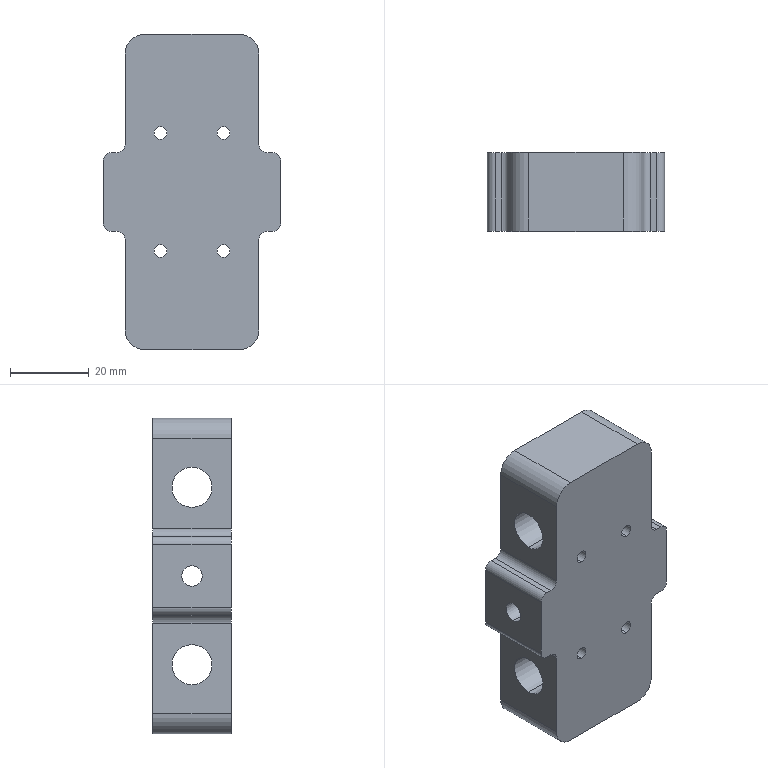Part | SolidWorks | features BaseBody 1 | 1 solid | 40 faces | box 45 x 20 x 80 mm | volume 51215 mm3 | cylinder 26 | plane 14 | commonest cylinder face diameters 3.2 x8 4 x8 10 x4 10.2 x4 5.2 x2
STEP:
#1=CARTESIAN_POINT('',(8.,20.,13.4));
#2=VERTEX_POINT('',#1);
#3=CARTESIAN_POINT('',(8.,20.,16.6));
#4=VERTEX_POINT('',#3);
#5=CARTESIAN_POINT('',(8.,20.,15.));
#6=DIRECTION('',(0.,1.,0.));
#7=DIRECTION('',(0.,0.,-1.));
#8=AXIS2_PLACEMENT_3D('',#5,#6,#7);
#9=CIRCLE('',#8,1.6);
#10=EDGE_CURVE('',#2,#4,#9,.T.);
#11=ORIENTED_EDGE('',*,*,#10,.T.);
#12=CARTESIAN_POINT('',(8.,0.,16.6));
#13=VERTEX_POINT('',#12);
#14=CARTESIAN_POINT('',(8.,20.,16.6));
#15=DIRECTION('',(0.,-1.,0.));
#16=VECTOR('',#15,1000.);
#17=LINE('',#14,#16);
#18=EDGE_CURVE('',#4,#13,#17,.T.);
#19=ORIENTED_EDGE('',*,*,#18,.T.);
#20=CARTESIAN_POINT('',(8.,0.,13.4));
#21=VERTEX_POINT('',#20);
#22=CARTESIAN_POINT('',(8.,0.,15.));
#23=DIRECTION('',(0.,1.,0.));
#24=DIRECTION('',(0.,0.,-1.));
#25=AXIS2_PLACEMENT_3D('',#22,#23,#24);
#26=CIRCLE('',#25,1.6);
#27=EDGE_CURVE('',#21,#13,#26,.T.);
#28=ORIENTED_EDGE('',*,*,#27,.F.);
#29=CARTESIAN_POINT('',(8.,20.,13.4));
#30=DIRECTION('',(0.,-1.,0.));
#31=VECTOR('',#30,1000.);
#32=LINE('',#29,#31);
#33=EDGE_CURVE('',#2,#21,#32,.T.);
#34=ORIENTED_EDGE('',*,*,#33,.F.);
#35=EDGE_LOOP('',(#11,#19,#28,#34));
#36=FACE_OUTER_BOUND('',#35,.T.);
#37=CARTESIAN_POINT('',(8.,20.,15.));
#38=DIRECTION('',(0.,-1.,0.));
#39=DIRECTION('',(0.,0.,-1.));
#40=AXIS2_PLACEMENT_3D('',#37,#38,#39);
#41=CYLINDRICAL_SURFACE('',#40,1.6);
#42=ADVANCED_FACE('',(#36),#41,.F.);
#43=CARTESIAN_POINT('',(-8.,20.,13.4));
#44=VERTEX_POINT('',#43);
#45=CARTESIAN_POINT('',(-8.,20.,16.6));
#46=VERTEX_POINT('',#45);
#47=CARTESIAN_POINT('',(-8.,20.,15.));
#48=DIRECTION('',(0.,1.,0.));
#49=DIRECTION('',(0.,0.,-1.));
#50=AXIS2_PLACEMENT_3D('',#47,#48,#49);
#51=CIRCLE('',#50,1.6);
#52=EDGE_CURVE('',#44,#46,#51,.T.);
#53=ORIENTED_EDGE('',*,*,#52,.T.);
#54=CARTESIAN_POINT('',(-8.,0.,16.6));
#55=VERTEX_POINT('',#54);
#56=CARTESIAN_POINT('',(-8.,20.,16.6));
#57=DIRECTION('',(0.,-1.,0.));
#58=VECTOR('',#57,1000.);
#59=LINE('',#56,#58);
#60=EDGE_CURVE('',#46,#55,#59,.T.);
#61=ORIENTED_EDGE('',*,*,#60,.T.);
#62=CARTESIAN_POINT('',(-8.,0.,13.4));
#63=VERTEX_POINT('',#62);
#64=CARTESIAN_POINT('',(-8.,0.,15.));
#65=DIRECTION('',(0.,1.,0.));
#66=DIRECTION('',(0.,0.,-1.));
#67=AXIS2_PLACEMENT_3D('',#64,#65,#66);
#68=CIRCLE('',#67,1.6);
#69=EDGE_CURVE('',#63,#55,#68,.T.);
#70=ORIENTED_EDGE('',*,*,#69,.F.);
#71=CARTESIAN_POINT('',(-8.,20.,13.4));
#72=DIRECTION('',(0.,-1.,0.));
#73=VECTOR('',#72,1000.);
#74=LINE('',#71,#73);
#75=EDGE_CURVE('',#44,#63,#74,.T.);
#76=ORIENTED_EDGE('',*,*,#75,.F.);
#77=EDGE_LOOP('',(#53,#61,#70,#76));
#78=FACE_OUTER_BOUND('',#77,.T.);
#79=CARTESIAN_POINT('',(-8.,20.,15.));
#80=DIRECTION('',(0.,-1.,0.));
#81=DIRECTION('',(0.,0.,-1.));
#82=AXIS2_PLACEMENT_3D('',#79,#80,#81);
#83=CYLINDRICAL_SURFACE('',#82,1.6);
#84=ADVANCED_FACE('',(#78),#83,.F.);
#85=CARTESIAN_POINT('',(-8.,20.,-16.6));
#86=VERTEX_POINT('',#85);
#87=CARTESIAN_POINT('',(-8.,20.,-13.4));
#88=VERTEX_POINT('',#87);
#89=CARTESIAN_POINT('',(-8.,20.,-15.));
#90=DIRECTION('',(0.,1.,0.));
#91=DIRECTION('',(0.,0.,-1.));
#92=AXIS2_PLACEMENT_3D('',#89,#90,#91);
#93=CIRCLE('',#92,1.6);
#94=EDGE_CURVE('',#86,#88,#93,.T.);
#95=ORIENTED_EDGE('',*,*,#94,.T.);
#96=CARTESIAN_POINT('',(-8.,0.,-13.4));
#97=VERTEX_POINT('',#96);
#98=CARTESIAN_POINT('',(-8.,20.,-13.4));
#99=DIRECTION('',(0.,-1.,0.));
#100=VECTOR('',#99,1000.);
#101=LINE('',#98,#100);
#102=EDGE_CURVE('',#88,#97,#101,.T.);
#103=ORIENTED_EDGE('',*,*,#102,.T.);
#104=CARTESIAN_POINT('',(-8.,0.,-16.6));
#105=VERTEX_POINT('',#104);
#106=CARTESIAN_POINT('',(-8.,0.,-15.));
#107=DIRECTION('',(0.,1.,0.));
#108=DIRECTION('',(0.,0.,-1.));
#109=AXIS2_PLACEMENT_3D('',#106,#107,#108);
#110=CIRCLE('',#109,1.6);
#111=EDGE_CURVE('',#105,#97,#110,.T.);
#112=ORIENTED_EDGE('',*,*,#111,.F.);
#113=CARTESIAN_POINT('',(-8.,20.,-16.6));
#114=DIRECTION('',(0.,-1.,0.));
#115=VECTOR('',#114,1000.);
#116=LINE('',#113,#115);
#117=EDGE_CURVE('',#86,#105,#116,.T.);
#118=ORIENTED_EDGE('',*,*,#117,.F.);
#119=EDGE_LOOP('',(#95,#103,#112,#118));
#120=FACE_OUTER_BOUND('',#119,.T.);
#121=CARTESIAN_POINT('',(-8.,20.,-15.));
#122=DIRECTION('',(0.,-1.,0.));
#123=DIRECTION('',(0.,0.,-1.));
#124=AXIS2_PLACEMENT_3D('',#121,#122,#123);
#125=CYLINDRICAL_SURFACE('',#124,1.6);
#126=ADVANCED_FACE('',(#120),#125,.F.);
#127=CARTESIAN_POINT('',(8.,20.,-16.6));
#128=VERTEX_POINT('',#127);
#129=CARTESIAN_POINT('',(8.,20.,-13.4));
#130=VERTEX_POINT('',#129);
#131=CARTESIAN_POINT('',(8.,20.,-15.));
#132=DIRECTION('',(0.,1.,0.));
#133=DIRECTION('',(0.,0.,-1.));
#134=AXIS2_PLACEMENT_3D('',#131,#132,#133);
#135=CIRCLE('',#134,1.6);
#136=EDGE_CURVE('',#128,#130,#135,.T.);
#137=ORIENTED_EDGE('',*,*,#136,.T.);
#138=CARTESIAN_POINT('',(8.,0.,-13.4));
#139=VERTEX_POINT('',#138);
#140=CARTESIAN_POINT('',(8.,20.,-13.4));
#141=DIRECTION('',(0.,-1.,0.));
#142=VECTOR('',#141,1000.);
#143=LINE('',#140,#142);
#144=EDGE_CURVE('',#130,#139,#143,.T.);
#145=ORIENTED_EDGE('',*,*,#144,.T.);
#146=CARTESIAN_POINT('',(8.,0.,-16.6));
#147=VERTEX_POINT('',#146);
#148=CARTESIAN_POINT('',(8.,0.,-15.));
#149=DIRECTION('',(0.,1.,0.));
#150=DIRECTION('',(0.,0.,-1.));
#151=AXIS2_PLACEMENT_3D('',#148,#149,#150);
#152=CIRCLE('',#151,1.6);
#153=EDGE_CURVE('',#147,#139,#152,.T.);
#154=ORIENTED_EDGE('',*,*,#153,.F.);
#155=CARTESIAN_POINT('',(8.,20.,-16.6));
#156=DIRECTION('',(0.,-1.,0.));
#157=VECTOR('',#156,1000.);
#158=LINE('',#155,#157);
#159=EDGE_CURVE('',#128,#147,#158,.T.);
#160=ORIENTED_EDGE('',*,*,#159,.F.);
#161=EDGE_LOOP('',(#137,#145,#154,#160));
#162=FACE_OUTER_BOUND('',#161,.T.);
#163=CARTESIAN_POINT('',(8.,20.,-15.));
#164=DIRECTION('',(0.,-1.,0.));
#165=DIRECTION('',(0.,0.,-1.));
#166=AXIS2_PLACEMENT_3D('',#163,#164,#165);
#167=CYLINDRICAL_SURFACE('',#166,1.6);
#168=ADVANCED_FACE('',(#162),#167,.F.);
#169=CARTESIAN_POINT('',(17.,10.,-17.4));
#170=VERTEX_POINT('',#169);
#171=CARTESIAN_POINT('',(17.,10.,-27.6));
#172=VERTEX_POINT('',#171);
#173=CARTESIAN_POINT('',(17.,10.,-22.5));
#174=DIRECTION('',(1.,0.,0.));
#175=DIRECTION('',(0.,0.,1.));
#176=AXIS2_PLACEMENT_3D('',#173,#174,#175);
#177=CIRCLE('',#176,5.1);
#178=EDGE_CURVE('',#170,#172,#177,.T.);
#179=ORIENTED_EDGE('',*,*,#178,.T.);
#180=CARTESIAN_POINT('',(-17.,10.,-27.6));
#181=VERTEX_POINT('',#180);
#182=CARTESIAN_POINT('',(22.5,10.,-27.6));
#183=DIRECTION('',(-1.,0.,0.));
#184=VECTOR('',#183,1000.);
#185=LINE('',#182,#184);
#186=EDGE_CURVE('',#172,#181,#185,.T.);
#187=ORIENTED_EDGE('',*,*,#186,.T.);
#188=CARTESIAN_POINT('',(-17.,10.,-17.4));
#189=VERTEX_POINT('',#188);
#190=CARTESIAN_POINT('',(-17.,10.,-22.5));
#191=DIRECTION('',(-1.,0.,0.));
#192=DIRECTION('',(0.,0.,1.));
#193=AXIS2_PLACEMENT_3D('',#190,#191,#192);
#194=CIRCLE('',#193,5.1);
#195=EDGE_CURVE('',#181,#189,#194,.T.);
#196=ORIENTED_EDGE('',*,*,#195,.T.);
#197=CARTESIAN_POINT('',(22.5,10.,-17.4));
#198=DIRECTION('',(-1.,0.,0.));
#199=VECTOR('',#198,1000.);
#200=LINE('',#197,#199);
#201=EDGE_CURVE('',#170,#189,#200,.T.);
#202=ORIENTED_EDGE('',*,*,#201,.F.);
#203=EDGE_LOOP('',(#179,#187,#196,#202));
#204=FACE_OUTER_BOUND('',#203,.T.);
#205=CARTESIAN_POINT('',(22.5,10.,-22.5));
#206=DIRECTION('',(-1.,0.,0.));
#207=DIRECTION('',(0.,0.,1.));
#208=AXIS2_PLACEMENT_3D('',#205,#206,#207);
#209=CYLINDRICAL_SURFACE('',#208,5.1);
#210=ADVANCED_FACE('',(#204),#209,.F.);
#211=CARTESIAN_POINT('',(22.5,10.,2.6));
#212=VERTEX_POINT('',#211);
#213=CARTESIAN_POINT('',(22.5,10.,-2.6));
#214=VERTEX_POINT('',#213);
#215=CARTESIAN_POINT('',(22.5,10.,0.));
#216=DIRECTION('',(1.,0.,0.));
#217=DIRECTION('',(0.,0.,1.));
#218=AXIS2_PLACEMENT_3D('',#215,#216,#217);
#219=CIRCLE('',#218,2.6);
#220=EDGE_CURVE('',#212,#214,#219,.T.);
#221=ORIENTED_EDGE('',*,*,#220,.T.);
#222=CARTESIAN_POINT('',(-22.5,10.,-2.6));
#223=VERTEX_POINT('',#222);
#224=CARTESIAN_POINT('',(22.5,10.,-2.6));
#225=DIRECTION('',(-1.,0.,0.));
#226=VECTOR('',#225,1000.);
#227=LINE('',#224,#226);
#228=EDGE_CURVE('',#214,#223,#227,.T.);
#229=ORIENTED_EDGE('',*,*,#228,.T.);
#230=CARTESIAN_POINT('',(-22.5,10.,2.6));
#231=VERTEX_POINT('',#230);
#232=CARTESIAN_POINT('',(-22.5,10.,0.));
#233=DIRECTION('',(-1.,0.,0.));
#234=DIRECTION('',(0.,0.,1.));
#235=AXIS2_PLACEMENT_3D('',#232,#233,#234);
#236=CIRCLE('',#235,2.6);
#237=EDGE_CURVE('',#223,#231,#236,.T.);
#238=ORIENTED_EDGE('',*,*,#237,.T.);
#239=CARTESIAN_POINT('',(22.5,10.,2.6));
#240=DIRECTION('',(-1.,0.,0.));
#241=VECTOR('',#240,1000.);
#242=LINE('',#239,#241);
#243=EDGE_CURVE('',#212,#231,#242,.T.);
#244=ORIENTED_EDGE('',*,*,#243,.F.);
#245=EDGE_LOOP('',(#221,#229,#238,#244));
#246=FACE_OUTER_BOUND('',#245,.T.);
#247=CARTESIAN_POINT('',(22.5,10.,0.));
#248=DIRECTION('',(-1.,0.,0.));
#249=DIRECTION('',(0.,0.,1.));
#250=AXIS2_PLACEMENT_3D('',#247,#248,#249);
#251=CYLINDRICAL_SURFACE('',#250,2.6);
#252=ADVANCED_FACE('',(#246),#251,.F.);
#253=CARTESIAN_POINT('',(17.,10.,27.6));
#254=VERTEX_POINT('',#253);
#255=CARTESIAN_POINT('',(17.,10.,17.4));
#256=VERTEX_POINT('',#255);
#257=CARTESIAN_POINT('',(17.,10.,22.5));
#258=DIRECTION('',(1.,0.,0.));
#259=DIRECTION('',(0.,0.,1.));
#260=AXIS2_PLACEMENT_3D('',#257,#258,#259);
#261=CIRCLE('',#260,5.1);
#262=EDGE_CURVE('',#254,#256,#261,.T.);
#263=ORIENTED_EDGE('',*,*,#262,.T.);
#264=CARTESIAN_POINT('',(-17.,10.,17.4));
#265=VERTEX_POINT('',#264);
#266=CARTESIAN_POINT('',(22.5,10.,17.4));
#267=DIRECTION('',(-1.,0.,0.));
#268=VECTOR('',#267,1000.);
#269=LINE('',#266,#268);
#270=EDGE_CURVE('',#256,#265,#269,.T.);
#271=ORIENTED_EDGE('',*,*,#270,.T.);
#272=CARTESIAN_POINT('',(-17.,10.,27.6));
#273=VERTEX_POINT('',#272);
#274=CARTESIAN_POINT('',(-17.,10.,22.5));
#275=DIRECTION('',(-1.,0.,0.));
#276=DIRECTION('',(0.,0.,1.));
#277=AXIS2_PLACEMENT_3D('',#274,#275,#276);
#278=CIRCLE('',#277,5.1);
#279=EDGE_CURVE('',#265,#273,#278,.T.);
#280=ORIENTED_EDGE('',*,*,#279,.T.);
#281=CARTESIAN_POINT('',(22.5,10.,27.6));
#282=DIRECTION('',(-1.,0.,0.));
#283=VECTOR('',#282,1000.);
#284=LINE('',#281,#283);
#285=EDGE_CURVE('',#254,#273,#284,.T.);
#286=ORIENTED_EDGE('',*,*,#285,.F.);
#287=EDGE_LOOP('',(#263,#271,#280,#286));
#288=FACE_OUTER_BOUND('',#287,.T.);
#289=CARTESIAN_POINT('',(22.5,10.,22.5));
#290=DIRECTION('',(-1.,0.,0.));
#291=DIRECTION('',(0.,0.,1.));
#292=AXIS2_PLACEMENT_3D('',#289,#290,#291);
#293=CYLINDRICAL_SURFACE('',#292,5.1);
#294=ADVANCED_FACE('',(#288),#293,.F.);
#295=CARTESIAN_POINT('',(12.,20.,-40.));
#296=VERTEX_POINT('',#295);
#297=CARTESIAN_POINT('',(17.,20.,-35.));
#298=VERTEX_POINT('',#297);
#299=CARTESIAN_POINT('',(12.,20.,-35.));
#300=DIRECTION('',(0.,-1.,0.));
#301=DIRECTION('',(0.,0.,1.));
#302=AXIS2_PLACEMENT_3D('',#299,#300,#301);
#303=CIRCLE('',#302,5.);
#304=EDGE_CURVE('',#296,#298,#303,.T.);
#305=ORIENTED_EDGE('',*,*,#304,.F.);
#306=CARTESIAN_POINT('',(-12.,20.,-40.));
#307=VERTEX_POINT('',#306);
#308=CARTESIAN_POINT('',(0.,20.,-40.));
#309=DIRECTION('',(1.,0.,0.));
#310=VECTOR('',#309,1000.);
#311=LINE('',#308,#310);
#312=EDGE_CURVE('',#307,#296,#311,.T.);
#313=ORIENTED_EDGE('',*,*,#312,.F.);
#314=CARTESIAN_POINT('',(-17.,20.,-35.));
#315=VERTEX_POINT('',#314);
#316=CARTESIAN_POINT('',(-12.,20.,-35.));
#317=DIRECTION('',(0.,-1.,0.));
#318=DIRECTION('',(0.,0.,1.));
#319=AXIS2_PLACEMENT_3D('',#316,#317,#318);
#320=CIRCLE('',#319,5.);
#321=EDGE_CURVE('',#315,#307,#320,.T.);
#322=ORIENTED_EDGE('',*,*,#321,.F.);
#323=CARTESIAN_POINT('',(-17.,20.,-12.));
#324=VERTEX_POINT('',#323);
#325=CARTESIAN_POINT('',(-17.,20.,0.));
#326=DIRECTION('',(0.,0.,-1.));
#327=VECTOR('',#326,1000.);
#328=LINE('',#325,#327);
#329=EDGE_CURVE('',#324,#315,#328,.T.);
#330=ORIENTED_EDGE('',*,*,#329,.F.);
#331=CARTESIAN_POINT('',(-19.,20.,-10.));
#332=VERTEX_POINT('',#331);
#333=CARTESIAN_POINT('',(-19.,20.,-12.));
#334=DIRECTION('',(0.,1.,0.));
#335=DIRECTION('',(0.,0.,-1.));
#336=AXIS2_PLACEMENT_3D('',#333,#334,#335);
#337=CIRCLE('',#336,2.);
#338=EDGE_CURVE('',#332,#324,#337,.T.);
#339=ORIENTED_EDGE('',*,*,#338,.F.);
#340=CARTESIAN_POINT('',(-20.5,20.,-10.));
#341=VERTEX_POINT('',#340);
#342=CARTESIAN_POINT('',(-17.,20.,-10.));
#343=DIRECTION('',(1.,0.,0.));
#344=VECTOR('',#343,1000.);
#345=LINE('',#342,#344);
#346=EDGE_CURVE('',#341,#332,#345,.T.);
#347=ORIENTED_EDGE('',*,*,#346,.F.);
#348=CARTESIAN_POINT('',(-22.5,20.,-8.));
#349=VERTEX_POINT('',#348);
#350=CARTESIAN_POINT('',(-20.5,20.,-8.));
#351=DIRECTION('',(0.,-1.,0.));
#352=DIRECTION('',(0.,0.,1.));
#353=AXIS2_PLACEMENT_3D('',#350,#351,#352);
#354=CIRCLE('',#353,2.);
#355=EDGE_CURVE('',#349,#341,#354,.T.);
#356=ORIENTED_EDGE('',*,*,#355,.F.);
#357=CARTESIAN_POINT('',(-22.5,20.,8.));
#358=VERTEX_POINT('',#357);
#359=CARTESIAN_POINT('',(-22.5,20.,0.));
#360=DIRECTION('',(0.,0.,-1.));
#361=VECTOR('',#360,1000.);
#362=LINE('',#359,#361);
#363=EDGE_CURVE('',#358,#349,#362,.T.);
#364=ORIENTED_EDGE('',*,*,#363,.F.);
#365=CARTESIAN_POINT('',(-20.5,20.,10.));
#366=VERTEX_POINT('',#365);
#367=CARTESIAN_POINT('',(-20.5,20.,8.));
#368=DIRECTION('',(0.,-1.,0.));
#369=DIRECTION('',(0.,0.,-1.));
#370=AXIS2_PLACEMENT_3D('',#367,#368,#369);
#371=CIRCLE('',#370,2.);
#372=EDGE_CURVE('',#366,#358,#371,.T.);
#373=ORIENTED_EDGE('',*,*,#372,.F.);
#374=CARTESIAN_POINT('',(-19.,20.,10.));
#375=VERTEX_POINT('',#374);
#376=CARTESIAN_POINT('',(-17.,20.,10.));
#377=DIRECTION('',(1.,0.,0.));
#378=VECTOR('',#377,1000.);
#379=LINE('',#376,#378);
#380=EDGE_CURVE('',#366,#375,#379,.T.);
#381=ORIENTED_EDGE('',*,*,#380,.T.);
#382=CARTESIAN_POINT('',(-17.,20.,12.));
#383=VERTEX_POINT('',#382);
#384=CARTESIAN_POINT('',(-19.,20.,12.));
#385=DIRECTION('',(0.,1.,0.));
#386=DIRECTION('',(0.,0.,1.));
#387=AXIS2_PLACEMENT_3D('',#384,#385,#386);
#388=CIRCLE('',#387,2.);
#389=EDGE_CURVE('',#383,#375,#388,.T.);
#390=ORIENTED_EDGE('',*,*,#389,.F.);
#391=CARTESIAN_POINT('',(-17.,20.,35.));
#392=VERTEX_POINT('',#391);
#393=CARTESIAN_POINT('',(-17.,20.,0.));
#394=DIRECTION('',(0.,0.,-1.));
#395=VECTOR('',#394,1000.);
#396=LINE('',#393,#395);
#397=EDGE_CURVE('',#392,#383,#396,.T.);
#398=ORIENTED_EDGE('',*,*,#397,.F.);
#399=CARTESIAN_POINT('',(-12.,20.,40.));
#400=VERTEX_POINT('',#399);
#401=CARTESIAN_POINT('',(-12.,20.,35.));
#402=DIRECTION('',(0.,-1.,0.));
#403=DIRECTION('',(0.,0.,1.));
#404=AXIS2_PLACEMENT_3D('',#401,#402,#403);
#405=CIRCLE('',#404,5.);
#406=EDGE_CURVE('',#400,#392,#405,.T.);
#407=ORIENTED_EDGE('',*,*,#406,.F.);
#408=CARTESIAN_POINT('',(12.,20.,40.));
#409=VERTEX_POINT('',#408);
#410=CARTESIAN_POINT('',(0.,20.,40.));
#411=DIRECTION('',(-1.,0.,0.));
#412=VECTOR('',#411,1000.);
#413=LINE('',#410,#412);
#414=EDGE_CURVE('',#409,#400,#413,.T.);
#415=ORIENTED_EDGE('',*,*,#414,.F.);
#416=CARTESIAN_POINT('',(17.,20.,35.));
#417=VERTEX_POINT('',#416);
#418=CARTESIAN_POINT('',(12.,20.,35.));
#419=DIRECTION('',(0.,-1.,0.));
#420=DIRECTION('',(0.,0.,1.));
#421=AXIS2_PLACEMENT_3D('',#418,#419,#420);
#422=CIRCLE('',#421,5.);
#423=EDGE_CURVE('',#417,#409,#422,.T.);
#424=ORIENTED_EDGE('',*,*,#423,.F.);
#425=CARTESIAN_POINT('',(17.,20.,12.));
#426=VERTEX_POINT('',#425);
#427=CARTESIAN_POINT('',(17.,20.,0.));
#428=DIRECTION('',(0.,0.,1.));
#429=VECTOR('',#428,1000.);
#430=LINE('',#427,#429);
#431=EDGE_CURVE('',#426,#417,#430,.T.);
#432=ORIENTED_EDGE('',*,*,#431,.F.);
#433=CARTESIAN_POINT('',(19.,20.,10.));
#434=VERTEX_POINT('',#433);
#435=CARTESIAN_POINT('',(19.,20.,12.));
#436=DIRECTION('',(0.,1.,0.));
#437=DIRECTION('',(0.,0.,-1.));
#438=AXIS2_PLACEMENT_3D('',#435,#436,#437);
#439=CIRCLE('',#438,2.);
#440=EDGE_CURVE('',#434,#426,#439,.T.);
#441=ORIENTED_EDGE('',*,*,#440,.F.);
#442=CARTESIAN_POINT('',(20.5,20.,10.));
#443=VERTEX_POINT('',#442);
#444=CARTESIAN_POINT('',(17.,20.,10.));
#445=DIRECTION('',(-1.,0.,0.));
#446=VECTOR('',#445,1000.);
#447=LINE('',#444,#446);
#448=EDGE_CURVE('',#443,#434,#447,.T.);
#449=ORIENTED_EDGE('',*,*,#448,.F.);
#450=CARTESIAN_POINT('',(22.5,20.,8.));
#451=VERTEX_POINT('',#450);
#452=CARTESIAN_POINT('',(20.5,20.,8.));
#453=DIRECTION('',(0.,-1.,0.));
#454=DIRECTION('',(0.,0.,1.));
#455=AXIS2_PLACEMENT_3D('',#452,#453,#454);
#456=CIRCLE('',#455,2.);
#457=EDGE_CURVE('',#451,#443,#456,.T.);
#458=ORIENTED_EDGE('',*,*,#457,.F.);
#459=CARTESIAN_POINT('',(22.5,20.,-8.));
#460=VERTEX_POINT('',#459);
#461=CARTESIAN_POINT('',(22.5,20.,0.));
#462=DIRECTION('',(0.,0.,1.));
#463=VECTOR('',#462,1000.);
#464=LINE('',#461,#463);
#465=EDGE_CURVE('',#460,#451,#464,.T.);
#466=ORIENTED_EDGE('',*,*,#465,.F.);
#467=CARTESIAN_POINT('',(20.5,20.,-10.));
#468=VERTEX_POINT('',#467);
#469=CARTESIAN_POINT('',(20.5,20.,-8.));
#470=DIRECTION('',(0.,-1.,0.));
#471=DIRECTION('',(0.,0.,-1.));
#472=AXIS2_PLACEMENT_3D('',#469,#470,#471);
#473=CIRCLE('',#472,2.);
#474=EDGE_CURVE('',#468,#460,#473,.T.);
#475=ORIENTED_EDGE('',*,*,#474,.F.);
#476=CARTESIAN_POINT('',(19.,20.,-10.));
#477=VERTEX_POINT('',#476);
#478=CARTESIAN_POINT('',(17.,20.,-10.));
#479=DIRECTION('',(-1.,0.,0.));
#480=VECTOR('',#479,1000.);
#481=LINE('',#478,#480);
#482=EDGE_CURVE('',#468,#477,#481,.T.);
#483=ORIENTED_EDGE('',*,*,#482,.T.);
#484=CARTESIAN_POINT('',(17.,20.,-12.));
#485=VERTEX_POINT('',#484);
#486=CARTESIAN_POINT('',(19.,20.,-12.));
#487=DIRECTION('',(0.,1.,0.));
#488=DIRECTION('',(0.,0.,1.));
#489=AXIS2_PLACEMENT_3D('',#486,#487,#488);
#490=CIRCLE('',#489,2.);
#491=EDGE_CURVE('',#485,#477,#490,.T.);
#492=ORIENTED_EDGE('',*,*,#491,.F.);
#493=CARTESIAN_POINT('',(17.,20.,0.));
#494=DIRECTION('',(0.,0.,1.));
#495=VECTOR('',#494,1000.);
#496=LINE('',#493,#495);
#497=EDGE_CURVE('',#298,#485,#496,.T.);
#498=ORIENTED_EDGE('',*,*,#497,.F.);
#499=EDGE_LOOP('',(#305,#313,#322,#330,#339,#347,#356,#364,#373,#381,#390,#398,#407,#415,#424,#432,#441,#449,#458,#466,#475,#483,#492,#498));
#500=FACE_OUTER_BOUND('',#499,.T.);
#501=ORIENTED_EDGE('',*,*,#10,.F.);
#502=CARTESIAN_POINT('',(8.,20.,15.));
#503=DIRECTION('',(0.,1.,0.));
#504=DIRECTION('',(0.,0.,-1.));
#505=AXIS2_PLACEMENT_3D('',#502,#503,#504);
#506=CIRCLE('',#505,1.6);
#507=EDGE_CURVE('',#4,#2,#506,.T.);
#508=ORIENTED_EDGE('',*,*,#507,.F.);
#509=EDGE_LOOP('',(#501,#508));
#510=FACE_BOUND('',#509,.T.);
#511=ORIENTED_EDGE('',*,*,#52,.F.);
#512=CARTESIAN_POINT('',(-8.,20.,15.));
#513=DIRECTION('',(0.,1.,0.));
#514=DIRECTION('',(0.,0.,-1.));
#515=AXIS2_PLACEMENT_3D('',#512,#513,#514);
#516=CIRCLE('',#515,1.6);
#517=EDGE_CURVE('',#46,#44,#516,.T.);
#518=ORIENTED_EDGE('',*,*,#517,.F.);
#519=EDGE_LOOP('',(#511,#518));
#520=FACE_BOUND('',#519,.T.);
#521=ORIENTED_EDGE('',*,*,#94,.F.);
#522=CARTESIAN_POINT('',(-8.,20.,-15.));
#523=DIRECTION('',(0.,1.,0.));
#524=DIRECTION('',(0.,0.,-1.));
#525=AXIS2_PLACEMENT_3D('',#522,#523,#524);
#526=CIRCLE('',#525,1.6);
#527=EDGE_CURVE('',#88,#86,#526,.T.);
#528=ORIENTED_EDGE('',*,*,#527,.F.);
#529=EDGE_LOOP('',(#521,#528));
#530=FACE_BOUND('',#529,.T.);
#531=ORIENTED_EDGE('',*,*,#136,.F.);
#532=CARTESIAN_POINT('',(8.,20.,-15.));
#533=DIRECTION('',(0.,1.,0.));
#534=DIRECTION('',(0.,0.,-1.));
#535=AXIS2_PLACEMENT_3D('',#532,#533,#534);
#536=CIRCLE('',#535,1.6);
#537=EDGE_CURVE('',#130,#128,#536,.T.);
#538=ORIENTED_EDGE('',*,*,#537,.F.);
#539=EDGE_LOOP('',(#531,#538));
#540=FACE_BOUND('',#539,.T.);
#541=CARTESIAN_POINT('',(0.,20.,0.));
#542=DIRECTION('',(0.,-1.,0.));
#543=DIRECTION('',(0.,0.,-1.));
#544=AXIS2_PLACEMENT_3D('',#541,#542,#543);
#545=PLANE('',#544);
#546=ADVANCED_FACE('',(#500,#510,#520,#530,#540),#545,.F.);
#547=ORIENTED_EDGE('',*,*,#178,.F.);
#548=CARTESIAN_POINT('',(17.,10.,-22.5));
#549=DIRECTION('',(1.,0.,0.));
#550=DIRECTION('',(0.,0.,1.));
#551=AXIS2_PLACEMENT_3D('',#548,#549,#550);
#552=CIRCLE('',#551,5.1);
#553=EDGE_CURVE('',#172,#170,#552,.T.);
#554=ORIENTED_EDGE('',*,*,#553,.F.);
#555=EDGE_LOOP('',(#547,#554));
#556=FACE_BOUND('',#555,.T.);
#557=CARTESIAN_POINT('',(17.,0.,-35.));
#558=VERTEX_POINT('',#557);
#559=CARTESIAN_POINT('',(17.,0.,-35.));
#560=DIRECTION('',(0.,-1.,0.));
#561=VECTOR('',#560,1000.);
#562=LINE('',#559,#561);
#563=EDGE_CURVE('',#298,#558,#562,.T.);
#564=ORIENTED_EDGE('',*,*,#563,.F.);
#565=ORIENTED_EDGE('',*,*,#497,.T.);
#566=CARTESIAN_POINT('',(17.,0.,-12.));
#567=VERTEX_POINT('',#566);
#568=CARTESIAN_POINT('',(17.,0.,-12.));
#569=DIRECTION('',(0.,1.,0.));
#570=VECTOR('',#569,1000.);
#571=LINE('',#568,#570);
#572=EDGE_CURVE('',#567,#485,#571,.T.);
#573=ORIENTED_EDGE('',*,*,#572,.F.);
#574=CARTESIAN_POINT('',(17.,0.,0.));
#575=DIRECTION('',(0.,0.,1.));
#576=VECTOR('',#575,1000.);
#577=LINE('',#574,#576);
#578=EDGE_CURVE('',#558,#567,#577,.T.);
#579=ORIENTED_EDGE('',*,*,#578,.F.);
#580=EDGE_LOOP('',(#564,#565,#573,#579));
#581=FACE_OUTER_BOUND('',#580,.T.);
#582=CARTESIAN_POINT('',(17.,0.,0.));
#583=DIRECTION('',(-1.,0.,0.));
#584=DIRECTION('',(0.,0.,1.));
#585=AXIS2_PLACEMENT_3D('',#582,#583,#584);
#586=PLANE('',#585);
#587=ADVANCED_FACE('',(#556,#581),#586,.F.);
#588=ORIENTED_EDGE('',*,*,#304,.T.);
#589=ORIENTED_EDGE('',*,*,#563,.T.);
#590=CARTESIAN_POINT('',(12.,0.,-40.));
#591=VERTEX_POINT('',#590);
#592=CARTESIAN_POINT('',(12.,0.,-35.));
#593=DIRECTION('',(0.,1.,0.));
#594=DIRECTION('',(0.,0.,1.));
#595=AXIS2_PLACEMENT_3D('',#592,#593,#594);
#596=CIRCLE('',#595,5.);
#597=EDGE_CURVE('',#558,#591,#596,.T.);
#598=ORIENTED_EDGE('',*,*,#597,.T.);
#599=CARTESIAN_POINT('',(12.,0.,-40.));
#600=DIRECTION('',(0.,1.,0.));
#601=VECTOR('',#600,1000.);
#602=LINE('',#599,#601);
#603=EDGE_CURVE('',#591,#296,#602,.T.);
#604=ORIENTED_EDGE('',*,*,#603,.T.);
#605=EDGE_LOOP('',(#588,#589,#598,#604));
#606=FACE_OUTER_BOUND('',#605,.T.);
#607=CARTESIAN_POINT('',(12.,0.,-35.));
#608=DIRECTION('',(0.,1.,0.));
#609=DIRECTION('',(0.,0.,1.));
#610=AXIS2_PLACEMENT_3D('',#607,#608,#609);
#611=CYLINDRICAL_SURFACE('',#610,5.);
#612=ADVANCED_FACE('',(#606),#611,.T.);
#613=ORIENTED_EDGE('',*,*,#603,.F.);
#614=CARTESIAN_POINT('',(-12.,0.,-40.));
#615=VERTEX_POINT('',#614);
#616=CARTESIAN_POINT('',(-22.5,0.,-40.));
#617=DIRECTION('',(1.,0.,0.));
#618=VECTOR('',#617,1000.);
#619=LINE('',#616,#618);
#620=EDGE_CURVE('',#615,#591,#619,.T.);
#621=ORIENTED_EDGE('',*,*,#620,.F.);
#622=CARTESIAN_POINT('',(-12.,20.,-40.));
#623=DIRECTION('',(0.,-1.,0.));
#624=VECTOR('',#623,1000.);
#625=LINE('',#622,#624);
#626=EDGE_CURVE('',#307,#615,#625,.T.);
#627=ORIENTED_EDGE('',*,*,#626,.F.);
#628=ORIENTED_EDGE('',*,*,#312,.T.);
#629=EDGE_LOOP('',(#613,#621,#627,#628));
#630=FACE_OUTER_BOUND('',#629,.T.);
#631=CARTESIAN_POINT('',(-22.5,20.,-40.));
#632=DIRECTION('',(0.,0.,1.));
#633=DIRECTION('',(1.,0.,0.));
#634=AXIS2_PLACEMENT_3D('',#631,#632,#633);
#635=PLANE('',#634);
#636=ADVANCED_FACE('',(#630),#635,.F.);
#637=ORIENTED_EDGE('',*,*,#321,.T.);
#638=ORIENTED_EDGE('',*,*,#626,.T.);
#639=CARTESIAN_POINT('',(-17.,0.,-35.));
#640=VERTEX_POINT('',#639);
#641=CARTESIAN_POINT('',(-12.,0.,-35.));
#642=DIRECTION('',(0.,1.,0.));
#643=DIRECTION('',(0.,0.,1.));
#644=AXIS2_PLACEMENT_3D('',#641,#642,#643);
#645=CIRCLE('',#644,5.);
#646=EDGE_CURVE('',#615,#640,#645,.T.);
#647=ORIENTED_EDGE('',*,*,#646,.T.);
#648=CARTESIAN_POINT('',(-17.,20.,-35.));
#649=DIRECTION('',(0.,1.,0.));
#650=VECTOR('',#649,1000.);
#651=LINE('',#648,#650);
#652=EDGE_CURVE('',#640,#315,#651,.T.);
#653=ORIENTED_EDGE('',*,*,#652,.T.);
#654=EDGE_LOOP('',(#637,#638,#647,#653));
#655=FACE_OUTER_BOUND('',#654,.T.);
#656=CARTESIAN_POINT('',(-12.,20.,-35.));
#657=DIRECTION('',(0.,1.,0.));
#658=DIRECTION('',(0.,0.,1.));
#659=AXIS2_PLACEMENT_3D('',#656,#657,#658);
#660=CYLINDRICAL_SURFACE('',#659,5.);
#661=ADVANCED_FACE('',(#655),#660,.T.);
#662=CARTESIAN_POINT('',(-17.,10.,-22.5));
#663=DIRECTION('',(-1.,0.,0.));
#664=DIRECTION('',(0.,0.,1.));
#665=AXIS2_PLACEMENT_3D('',#662,#663,#664);
#666=CIRCLE('',#665,5.1);
#667=EDGE_CURVE('',#189,#181,#666,.T.);
#668=ORIENTED_EDGE('',*,*,#667,.F.);
#669=ORIENTED_EDGE('',*,*,#195,.F.);
#670=EDGE_LOOP('',(#668,#669));
#671=FACE_BOUND('',#670,.T.);
#672=ORIENTED_EDGE('',*,*,#652,.F.);
#673=CARTESIAN_POINT('',(-17.,0.,-12.));
#674=VERTEX_POINT('',#673);
#675=CARTESIAN_POINT('',(-17.,0.,0.));
#676=DIRECTION('',(0.,0.,-1.));
#677=VECTOR('',#676,1000.);
#678=LINE('',#675,#677);
#679=EDGE_CURVE('',#674,#640,#678,.T.);
#680=ORIENTED_EDGE('',*,*,#679,.F.);
#681=CARTESIAN_POINT('',(-17.,0.,-12.));
#682=DIRECTION('',(0.,-1.,0.));
#683=VECTOR('',#682,1000.);
#684=LINE('',#681,#683);
#685=EDGE_CURVE('',#324,#674,#684,.T.);
#686=ORIENTED_EDGE('',*,*,#685,.F.);
#687=ORIENTED_EDGE('',*,*,#329,.T.);
#688=EDGE_LOOP('',(#672,#680,#686,#687));
#689=FACE_OUTER_BOUND('',#688,.T.);
#690=CARTESIAN_POINT('',(-17.,0.,0.));
#691=DIRECTION('',(1.,0.,0.));
#692=DIRECTION('',(0.,0.,-1.));
#693=AXIS2_PLACEMENT_3D('',#690,#691,#692);
#694=PLANE('',#693);
#695=ADVANCED_FACE('',(#671,#689),#694,.F.);
#696=ORIENTED_EDGE('',*,*,#685,.T.);
#697=CARTESIAN_POINT('',(-19.,0.,-10.));
#698=VERTEX_POINT('',#697);
#699=CARTESIAN_POINT('',(-19.,0.,-12.));
#700=DIRECTION('',(0.,1.,0.));
#701=DIRECTION('',(0.,0.,-1.));
#702=AXIS2_PLACEMENT_3D('',#699,#700,#701);
#703=CIRCLE('',#702,2.);
#704=EDGE_CURVE('',#698,#674,#703,.T.);
#705=ORIENTED_EDGE('',*,*,#704,.F.);
#706=CARTESIAN_POINT('',(-19.,20.,-10.));
#707=DIRECTION('',(0.,-1.,0.));
#708=VECTOR('',#707,1000.);
#709=LINE('',#706,#708);
#710=EDGE_CURVE('',#332,#698,#709,.T.);
#711=ORIENTED_EDGE('',*,*,#710,.F.);
#712=ORIENTED_EDGE('',*,*,#338,.T.);
#713=EDGE_LOOP('',(#696,#705,#711,#712));
#714=FACE_OUTER_BOUND('',#713,.T.);
#715=CARTESIAN_POINT('',(-19.,20.,-12.));
#716=DIRECTION('',(0.,-1.,0.));
#717=DIRECTION('',(0.,0.,-1.));
#718=AXIS2_PLACEMENT_3D('',#715,#716,#717);
#719=CYLINDRICAL_SURFACE('',#718,2.);
#720=ADVANCED_FACE('',(#714),#719,.F.);
#721=CARTESIAN_POINT('',(-20.5,0.,-10.));
#722=VERTEX_POINT('',#721);
#723=CARTESIAN_POINT('',(-22.5,0.,-8.));
#724=VERTEX_POINT('',#723);
#725=CARTESIAN_POINT('',(-20.5,0.,-8.));
#726=DIRECTION('',(0.,1.,0.));
#727=DIRECTION('',(0.,0.,1.));
#728=AXIS2_PLACEMENT_3D('',#725,#726,#727);
#729=CIRCLE('',#728,2.);
#730=EDGE_CURVE('',#722,#724,#729,.T.);
#731=ORIENTED_EDGE('',*,*,#730,.T.);
#732=CARTESIAN_POINT('',(-22.5,20.,-8.));
#733=DIRECTION('',(0.,1.,0.));
#734=VECTOR('',#733,1000.);
#735=LINE('',#732,#734);
#736=EDGE_CURVE('',#724,#349,#735,.T.);
#737=ORIENTED_EDGE('',*,*,#736,.T.);
#738=ORIENTED_EDGE('',*,*,#355,.T.);
#739=CARTESIAN_POINT('',(-20.5,20.,-10.));
#740=DIRECTION('',(0.,-1.,0.));
#741=VECTOR('',#740,1000.);
#742=LINE('',#739,#741);
#743=EDGE_CURVE('',#341,#722,#742,.T.);
#744=ORIENTED_EDGE('',*,*,#743,.T.);
#745=EDGE_LOOP('',(#731,#737,#738,#744));
#746=FACE_OUTER_BOUND('',#745,.T.);
#747=CARTESIAN_POINT('',(-20.5,20.,-8.));
#748=DIRECTION('',(0.,1.,0.));
#749=DIRECTION('',(0.,0.,1.));
#750=AXIS2_PLACEMENT_3D('',#747,#748,#749);
#751=CYLINDRICAL_SURFACE('',#750,2.);
#752=ADVANCED_FACE('',(#746),#751,.T.);
#753=ORIENTED_EDGE('',*,*,#736,.F.);
#754=CARTESIAN_POINT('',(-22.5,0.,8.));
#755=VERTEX_POINT('',#754);
#756=CARTESIAN_POINT('',(-22.5,0.,40.));
#757=DIRECTION('',(0.,0.,-1.));
#758=VECTOR('',#757,1000.);
#759=LINE('',#756,#758);
#760=EDGE_CURVE('',#755,#724,#759,.T.);
#761=ORIENTED_EDGE('',*,*,#760,.F.);
#762=CARTESIAN_POINT('',(-22.5,20.,8.));
#763=DIRECTION('',(0.,-1.,0.));
#764=VECTOR('',#763,1000.);
#765=LINE('',#762,#764);
#766=EDGE_CURVE('',#358,#755,#765,.T.);
#767=ORIENTED_EDGE('',*,*,#766,.F.);
#768=ORIENTED_EDGE('',*,*,#363,.T.);
#769=EDGE_LOOP('',(#753,#761,#767,#768));
#770=FACE_OUTER_BOUND('',#769,.T.);
#771=CARTESIAN_POINT('',(-22.5,10.,0.));
#772=DIRECTION('',(-1.,0.,0.));
#773=DIRECTION('',(0.,0.,1.));
#774=AXIS2_PLACEMENT_3D('',#771,#772,#773);
#775=CIRCLE('',#774,2.6);
#776=EDGE_CURVE('',#231,#223,#775,.T.);
#777=ORIENTED_EDGE('',*,*,#776,.F.);
#778=ORIENTED_EDGE('',*,*,#237,.F.);
#779=EDGE_LOOP('',(#777,#778));
#780=FACE_BOUND('',#779,.T.);
#781=CARTESIAN_POINT('',(-22.5,20.,40.));
#782=DIRECTION('',(1.,0.,0.));
#783=DIRECTION('',(0.,0.,-1.));
#784=AXIS2_PLACEMENT_3D('',#781,#782,#783);
#785=PLANE('',#784);
#786=ADVANCED_FACE('',(#770,#780),#785,.F.);
#787=CARTESIAN_POINT('',(-20.5,0.,10.));
#788=VERTEX_POINT('',#787);
#789=CARTESIAN_POINT('',(-20.5,0.,8.));
#790=DIRECTION('',(0.,1.,0.));
#791=DIRECTION('',(0.,0.,-1.));
#792=AXIS2_PLACEMENT_3D('',#789,#790,#791);
#793=CIRCLE('',#792,2.);
#794=EDGE_CURVE('',#755,#788,#793,.T.);
#795=ORIENTED_EDGE('',*,*,#794,.T.);
#796=CARTESIAN_POINT('',(-20.5,20.,10.));
#797=DIRECTION('',(0.,1.,0.));
#798=VECTOR('',#797,1000.);
#799=LINE('',#796,#798);
#800=EDGE_CURVE('',#788,#366,#799,.T.);
#801=ORIENTED_EDGE('',*,*,#800,.T.);
#802=ORIENTED_EDGE('',*,*,#372,.T.);
#803=ORIENTED_EDGE('',*,*,#766,.T.);
#804=EDGE_LOOP('',(#795,#801,#802,#803));
#805=FACE_OUTER_BOUND('',#804,.T.);
#806=CARTESIAN_POINT('',(-20.5,20.,8.));
#807=DIRECTION('',(0.,-1.,0.));
#808=DIRECTION('',(0.,0.,-1.));
#809=AXIS2_PLACEMENT_3D('',#806,#807,#808);
#810=CYLINDRICAL_SURFACE('',#809,2.);
#811=ADVANCED_FACE('',(#805),#810,.T.);
#812=CARTESIAN_POINT('',(-19.,0.,10.));
#813=VERTEX_POINT('',#812);
#814=CARTESIAN_POINT('',(-19.,0.,10.));
#815=DIRECTION('',(0.,1.,0.));
#816=VECTOR('',#815,1000.);
#817=LINE('',#814,#816);
#818=EDGE_CURVE('',#813,#375,#817,.T.);
#819=ORIENTED_EDGE('',*,*,#818,.F.);
#820=CARTESIAN_POINT('',(-17.,0.,12.));
#821=VERTEX_POINT('',#820);
#822=CARTESIAN_POINT('',(-19.,0.,12.));
#823=DIRECTION('',(0.,1.,0.));
#824=DIRECTION('',(0.,0.,1.));
#825=AXIS2_PLACEMENT_3D('',#822,#823,#824);
#826=CIRCLE('',#825,2.);
#827=EDGE_CURVE('',#821,#813,#826,.T.);
#828=ORIENTED_EDGE('',*,*,#827,.F.);
#829=CARTESIAN_POINT('',(-17.,0.,12.));
#830=DIRECTION('',(0.,-1.,0.));
#831=VECTOR('',#830,1000.);
#832=LINE('',#829,#831);
#833=EDGE_CURVE('',#383,#821,#832,.T.);
#834=ORIENTED_EDGE('',*,*,#833,.F.);
#835=ORIENTED_EDGE('',*,*,#389,.T.);
#836=EDGE_LOOP('',(#819,#828,#834,#835));
#837=FACE_OUTER_BOUND('',#836,.T.);
#838=CARTESIAN_POINT('',(-19.,0.,12.));
#839=DIRECTION('',(0.,1.,0.));
#840=DIRECTION('',(0.,0.,1.));
#841=AXIS2_PLACEMENT_3D('',#838,#839,#840);
#842=CYLINDRICAL_SURFACE('',#841,2.);
#843=ADVANCED_FACE('',(#837),#842,.F.);
#844=CARTESIAN_POINT('',(-17.,10.,22.5));
#845=DIRECTION('',(-1.,0.,0.));
#846=DIRECTION('',(0.,0.,1.));
#847=AXIS2_PLACEMENT_3D('',#844,#845,#846);
#848=CIRCLE('',#847,5.1);
#849=EDGE_CURVE('',#273,#265,#848,.T.);
#850=ORIENTED_EDGE('',*,*,#849,.F.);
#851=ORIENTED_EDGE('',*,*,#279,.F.);
#852=EDGE_LOOP('',(#850,#851));
#853=FACE_BOUND('',#852,.T.);
#854=CARTESIAN_POINT('',(-17.,0.,35.));
#855=VERTEX_POINT('',#854);
#856=CARTESIAN_POINT('',(-17.,0.,35.));
#857=DIRECTION('',(0.,-1.,0.));
#858=VECTOR('',#857,1000.);
#859=LINE('',#856,#858);
#860=EDGE_CURVE('',#392,#855,#859,.T.);
#861=ORIENTED_EDGE('',*,*,#860,.F.);
#862=ORIENTED_EDGE('',*,*,#397,.T.);
#863=ORIENTED_EDGE('',*,*,#833,.T.);
#864=CARTESIAN_POINT('',(-17.,0.,0.));
#865=DIRECTION('',(0.,0.,-1.));
#866=VECTOR('',#865,1000.);
#867=LINE('',#864,#866);
#868=EDGE_CURVE('',#855,#821,#867,.T.);
#869=ORIENTED_EDGE('',*,*,#868,.F.);
#870=EDGE_LOOP('',(#861,#862,#863,#869));
#871=FACE_OUTER_BOUND('',#870,.T.);
#872=CARTESIAN_POINT('',(-17.,0.,0.));
#873=DIRECTION('',(1.,0.,0.));
#874=DIRECTION('',(0.,0.,-1.));
#875=AXIS2_PLACEMENT_3D('',#872,#873,#874);
#876=PLANE('',#875);
#877=ADVANCED_FACE('',(#853,#871),#876,.F.);
#878=ORIENTED_EDGE('',*,*,#406,.T.);
#879=ORIENTED_EDGE('',*,*,#860,.T.);
#880=CARTESIAN_POINT('',(-12.,0.,40.));
#881=VERTEX_POINT('',#880);
#882=CARTESIAN_POINT('',(-12.,0.,35.));
#883=DIRECTION('',(0.,1.,0.));
#884=DIRECTION('',(0.,0.,1.));
#885=AXIS2_PLACEMENT_3D('',#882,#883,#884);
#886=CIRCLE('',#885,5.);
#887=EDGE_CURVE('',#855,#881,#886,.T.);
#888=ORIENTED_EDGE('',*,*,#887,.T.);
#889=CARTESIAN_POINT('',(-12.,0.,40.));
#890=DIRECTION('',(0.,1.,0.));
#891=VECTOR('',#890,1000.);
#892=LINE('',#889,#891);
#893=EDGE_CURVE('',#881,#400,#892,.T.);
#894=ORIENTED_EDGE('',*,*,#893,.T.);
#895=EDGE_LOOP('',(#878,#879,#888,#894));
#896=FACE_OUTER_BOUND('',#895,.T.);
#897=CARTESIAN_POINT('',(-12.,0.,35.));
#898=DIRECTION('',(0.,1.,0.));
#899=DIRECTION('',(0.,0.,1.));
#900=AXIS2_PLACEMENT_3D('',#897,#898,#899);
#901=CYLINDRICAL_SURFACE('',#900,5.);
#902=ADVANCED_FACE('',(#896),#901,.T.);
#903=CARTESIAN_POINT('',(12.,0.,40.));
#904=VERTEX_POINT('',#903);
#905=CARTESIAN_POINT('',(12.,20.,40.));
#906=DIRECTION('',(0.,-1.,0.));
#907=VECTOR('',#906,1000.);
#908=LINE('',#905,#907);
#909=EDGE_CURVE('',#409,#904,#908,.T.);
#910=ORIENTED_EDGE('',*,*,#909,.F.);
#911=ORIENTED_EDGE('',*,*,#414,.T.);
#912=ORIENTED_EDGE('',*,*,#893,.F.);
#913=CARTESIAN_POINT('',(-22.5,0.,40.));
#914=DIRECTION('',(-1.,0.,0.));
#915=VECTOR('',#914,1000.);
#916=LINE('',#913,#915);
#917=EDGE_CURVE('',#904,#881,#916,.T.);
#918=ORIENTED_EDGE('',*,*,#917,.F.);
#919=EDGE_LOOP('',(#910,#911,#912,#918));
#920=FACE_OUTER_BOUND('',#919,.T.);
#921=CARTESIAN_POINT('',(-22.5,20.,40.));
#922=DIRECTION('',(0.,0.,-1.));
#923=DIRECTION('',(-1.,0.,0.));
#924=AXIS2_PLACEMENT_3D('',#921,#922,#923);
#925=PLANE('',#924);
#926=ADVANCED_FACE('',(#920),#925,.F.);
#927=ORIENTED_EDGE('',*,*,#423,.T.);
#928=ORIENTED_EDGE('',*,*,#909,.T.);
#929=CARTESIAN_POINT('',(17.,0.,35.));
#930=VERTEX_POINT('',#929);
#931=CARTESIAN_POINT('',(12.,0.,35.));
#932=DIRECTION('',(0.,1.,0.));
#933=DIRECTION('',(0.,0.,1.));
#934=AXIS2_PLACEMENT_3D('',#931,#932,#933);
#935=CIRCLE('',#934,5.);
#936=EDGE_CURVE('',#904,#930,#935,.T.);
#937=ORIENTED_EDGE('',*,*,#936,.T.);
#938=CARTESIAN_POINT('',(17.,20.,35.));
#939=DIRECTION('',(0.,1.,0.));
#940=VECTOR('',#939,1000.);
#941=LINE('',#938,#940);
#942=EDGE_CURVE('',#930,#417,#941,.T.);
#943=ORIENTED_EDGE('',*,*,#942,.T.);
#944=EDGE_LOOP('',(#927,#928,#937,#943));
#945=FACE_OUTER_BOUND('',#944,.T.);
#946=CARTESIAN_POINT('',(12.,20.,35.));
#947=DIRECTION('',(0.,1.,0.));
#948=DIRECTION('',(0.,0.,1.));
#949=AXIS2_PLACEMENT_3D('',#946,#947,#948);
#950=CYLINDRICAL_SURFACE('',#949,5.);
#951=ADVANCED_FACE('',(#945),#950,.T.);
#952=ORIENTED_EDGE('',*,*,#262,.F.);
#953=CARTESIAN_POINT('',(17.,10.,22.5));
#954=DIRECTION('',(1.,0.,0.));
#955=DIRECTION('',(0.,0.,1.));
#956=AXIS2_PLACEMENT_3D('',#953,#954,#955);
#957=CIRCLE('',#956,5.1);
#958=EDGE_CURVE('',#256,#254,#957,.T.);
#959=ORIENTED_EDGE('',*,*,#958,.F.);
#960=EDGE_LOOP('',(#952,#959));
#961=FACE_BOUND('',#960,.T.);
#962=ORIENTED_EDGE('',*,*,#942,.F.);
#963=CARTESIAN_POINT('',(17.,0.,12.));
#964=VERTEX_POINT('',#963);
#965=CARTESIAN_POINT('',(17.,0.,0.));
#966=DIRECTION('',(0.,0.,1.));
#967=VECTOR('',#966,1000.);
#968=LINE('',#965,#967);
#969=EDGE_CURVE('',#964,#930,#968,.T.);
#970=ORIENTED_EDGE('',*,*,#969,.F.);
#971=CARTESIAN_POINT('',(17.,0.,12.));
#972=DIRECTION('',(0.,-1.,0.));
#973=VECTOR('',#972,1000.);
#974=LINE('',#971,#973);
#975=EDGE_CURVE('',#426,#964,#974,.T.);
#976=ORIENTED_EDGE('',*,*,#975,.F.);
#977=ORIENTED_EDGE('',*,*,#431,.T.);
#978=EDGE_LOOP('',(#962,#970,#976,#977));
#979=FACE_OUTER_BOUND('',#978,.T.);
#980=CARTESIAN_POINT('',(17.,0.,0.));
#981=DIRECTION('',(-1.,0.,0.));
#982=DIRECTION('',(0.,0.,1.));
#983=AXIS2_PLACEMENT_3D('',#980,#981,#982);
#984=PLANE('',#983);
#985=ADVANCED_FACE('',(#961,#979),#984,.F.);
#986=ORIENTED_EDGE('',*,*,#975,.T.);
#987=CARTESIAN_POINT('',(19.,0.,10.));
#988=VERTEX_POINT('',#987);
#989=CARTESIAN_POINT('',(19.,0.,12.));
#990=DIRECTION('',(0.,1.,0.));
#991=DIRECTION('',(0.,0.,-1.));
#992=AXIS2_PLACEMENT_3D('',#989,#990,#991);
#993=CIRCLE('',#992,2.);
#994=EDGE_CURVE('',#988,#964,#993,.T.);
#995=ORIENTED_EDGE('',*,*,#994,.F.);
#996=CARTESIAN_POINT('',(19.,20.,10.));
#997=DIRECTION('',(0.,-1.,0.));
#998=VECTOR('',#997,1000.);
#999=LINE('',#996,#998);
#1000=EDGE_CURVE('',#434,#988,#999,.T.);
#1001=ORIENTED_EDGE('',*,*,#1000,.F.);
#1002=ORIENTED_EDGE('',*,*,#440,.T.);
#1003=EDGE_LOOP('',(#986,#995,#1001,#1002));
#1004=FACE_OUTER_BOUND('',#1003,.T.);
#1005=CARTESIAN_POINT('',(19.,20.,12.));
#1006=DIRECTION('',(0.,-1.,0.));
#1007=DIRECTION('',(0.,0.,-1.));
#1008=AXIS2_PLACEMENT_3D('',#1005,#1006,#1007);
#1009=CYLINDRICAL_SURFACE('',#1008,2.);
#1010=ADVANCED_FACE('',(#1004),#1009,.F.);
#1011=CARTESIAN_POINT('',(20.5,0.,10.));
#1012=VERTEX_POINT('',#1011);
#1013=CARTESIAN_POINT('',(22.5,0.,8.));
#1014=VERTEX_POINT('',#1013);
#1015=CARTESIAN_POINT('',(20.5,0.,8.));
#1016=DIRECTION('',(0.,1.,0.));
#1017=DIRECTION('',(0.,0.,1.));
#1018=AXIS2_PLACEMENT_3D('',#1015,#1016,#1017);
#1019=CIRCLE('',#1018,2.);
#1020=EDGE_CURVE('',#1012,#1014,#1019,.T.);
#1021=ORIENTED_EDGE('',*,*,#1020,.T.);
#1022=CARTESIAN_POINT('',(22.5,20.,8.));
#1023=DIRECTION('',(0.,1.,0.));
#1024=VECTOR('',#1023,1000.);
#1025=LINE('',#1022,#1024);
#1026=EDGE_CURVE('',#1014,#451,#1025,.T.);
#1027=ORIENTED_EDGE('',*,*,#1026,.T.);
#1028=ORIENTED_EDGE('',*,*,#457,.T.);
#1029=CARTESIAN_POINT('',(20.5,20.,10.));
#1030=DIRECTION('',(0.,-1.,0.));
#1031=VECTOR('',#1030,1000.);
#1032=LINE('',#1029,#1031);
#1033=EDGE_CURVE('',#443,#1012,#1032,.T.);
#1034=ORIENTED_EDGE('',*,*,#1033,.T.);
#1035=EDGE_LOOP('',(#1021,#1027,#1028,#1034));
#1036=FACE_OUTER_BOUND('',#1035,.T.);
#1037=CARTESIAN_POINT('',(20.5,20.,8.));
#1038=DIRECTION('',(0.,1.,0.));
#1039=DIRECTION('',(0.,0.,1.));
#1040=AXIS2_PLACEMENT_3D('',#1037,#1038,#1039);
#1041=CYLINDRICAL_SURFACE('',#1040,2.);
#1042=ADVANCED_FACE('',(#1036),#1041,.T.);
#1043=CARTESIAN_POINT('',(22.5,0.,-8.));
#1044=VERTEX_POINT('',#1043);
#1045=CARTESIAN_POINT('',(22.5,20.,-8.));
#1046=DIRECTION('',(0.,-1.,0.));
#1047=VECTOR('',#1046,1000.);
#1048=LINE('',#1045,#1047);
#1049=EDGE_CURVE('',#460,#1044,#1048,.T.);
#1050=ORIENTED_EDGE('',*,*,#1049,.F.);
#1051=ORIENTED_EDGE('',*,*,#465,.T.);
#1052=ORIENTED_EDGE('',*,*,#1026,.F.);
#1053=CARTESIAN_POINT('',(22.5,0.,40.));
#1054=DIRECTION('',(0.,0.,1.));
#1055=VECTOR('',#1054,1000.);
#1056=LINE('',#1053,#1055);
#1057=EDGE_CURVE('',#1044,#1014,#1056,.T.);
#1058=ORIENTED_EDGE('',*,*,#1057,.F.);
#1059=EDGE_LOOP('',(#1050,#1051,#1052,#1058));
#1060=FACE_OUTER_BOUND('',#1059,.T.);
#1061=ORIENTED_EDGE('',*,*,#220,.F.);
#1062=CARTESIAN_POINT('',(22.5,10.,0.));
#1063=DIRECTION('',(1.,0.,0.));
#1064=DIRECTION('',(0.,0.,1.));
#1065=AXIS2_PLACEMENT_3D('',#1062,#1063,#1064);
#1066=CIRCLE('',#1065,2.6);
#1067=EDGE_CURVE('',#214,#212,#1066,.T.);
#1068=ORIENTED_EDGE('',*,*,#1067,.F.);
#1069=EDGE_LOOP('',(#1061,#1068));
#1070=FACE_BOUND('',#1069,.T.);
#1071=CARTESIAN_POINT('',(22.5,20.,40.));
#1072=DIRECTION('',(-1.,0.,0.));
#1073=DIRECTION('',(0.,0.,1.));
#1074=AXIS2_PLACEMENT_3D('',#1071,#1072,#1073);
#1075=PLANE('',#1074);
#1076=ADVANCED_FACE('',(#1060,#1070),#1075,.F.);
#1077=CARTESIAN_POINT('',(20.5,0.,-10.));
#1078=VERTEX_POINT('',#1077);
#1079=CARTESIAN_POINT('',(20.5,0.,-8.));
#1080=DIRECTION('',(0.,1.,0.));
#1081=DIRECTION('',(0.,0.,-1.));
#1082=AXIS2_PLACEMENT_3D('',#1079,#1080,#1081);
#1083=CIRCLE('',#1082,2.);
#1084=EDGE_CURVE('',#1044,#1078,#1083,.T.);
#1085=ORIENTED_EDGE('',*,*,#1084,.T.);
#1086=CARTESIAN_POINT('',(20.5,20.,-10.));
#1087=DIRECTION('',(0.,1.,0.));
#1088=VECTOR('',#1087,1000.);
#1089=LINE('',#1086,#1088);
#1090=EDGE_CURVE('',#1078,#468,#1089,.T.);
#1091=ORIENTED_EDGE('',*,*,#1090,.T.);
#1092=ORIENTED_EDGE('',*,*,#474,.T.);
#1093=ORIENTED_EDGE('',*,*,#1049,.T.);
#1094=EDGE_LOOP('',(#1085,#1091,#1092,#1093));
#1095=FACE_OUTER_BOUND('',#1094,.T.);
#1096=CARTESIAN_POINT('',(20.5,20.,-8.));
#1097=DIRECTION('',(0.,-1.,0.));
#1098=DIRECTION('',(0.,0.,-1.));
#1099=AXIS2_PLACEMENT_3D('',#1096,#1097,#1098);
#1100=CYLINDRICAL_SURFACE('',#1099,2.);
#1101=ADVANCED_FACE('',(#1095),#1100,.T.);
#1102=CARTESIAN_POINT('',(19.,0.,-10.));
#1103=VERTEX_POINT('',#1102);
#1104=CARTESIAN_POINT('',(19.,0.,-10.));
#1105=DIRECTION('',(0.,1.,0.));
#1106=VECTOR('',#1105,1000.);
#1107=LINE('',#1104,#1106);
#1108=EDGE_CURVE('',#1103,#477,#1107,.T.);
#1109=ORIENTED_EDGE('',*,*,#1108,.F.);
#1110=CARTESIAN_POINT('',(19.,0.,-12.));
#1111=DIRECTION('',(0.,1.,0.));
#1112=DIRECTION('',(0.,0.,1.));
#1113=AXIS2_PLACEMENT_3D('',#1110,#1111,#1112);
#1114=CIRCLE('',#1113,2.);
#1115=EDGE_CURVE('',#567,#1103,#1114,.T.);
#1116=ORIENTED_EDGE('',*,*,#1115,.F.);
#1117=ORIENTED_EDGE('',*,*,#572,.T.);
#1118=ORIENTED_EDGE('',*,*,#491,.T.);
#1119=EDGE_LOOP('',(#1109,#1116,#1117,#1118));
#1120=FACE_OUTER_BOUND('',#1119,.T.);
#1121=CARTESIAN_POINT('',(19.,0.,-12.));
#1122=DIRECTION('',(0.,1.,0.));
#1123=DIRECTION('',(0.,0.,1.));
#1124=AXIS2_PLACEMENT_3D('',#1121,#1122,#1123);
#1125=CYLINDRICAL_SURFACE('',#1124,2.);
#1126=ADVANCED_FACE('',(#1120),#1125,.F.);
#1127=ORIENTED_EDGE('',*,*,#18,.F.);
#1128=ORIENTED_EDGE('',*,*,#507,.T.);
#1129=ORIENTED_EDGE('',*,*,#33,.T.);
#1130=CARTESIAN_POINT('',(8.,0.,15.));
#1131=DIRECTION('',(0.,1.,0.));
#1132=DIRECTION('',(0.,0.,-1.));
#1133=AXIS2_PLACEMENT_3D('',#1130,#1131,#1132);
#1134=CIRCLE('',#1133,1.6);
#1135=EDGE_CURVE('',#13,#21,#1134,.T.);
#1136=ORIENTED_EDGE('',*,*,#1135,.F.);
#1137=EDGE_LOOP('',(#1127,#1128,#1129,#1136));
#1138=FACE_OUTER_BOUND('',#1137,.T.);
#1139=CARTESIAN_POINT('',(8.,20.,15.));
#1140=DIRECTION('',(0.,-1.,0.));
#1141=DIRECTION('',(0.,0.,-1.));
#1142=AXIS2_PLACEMENT_3D('',#1139,#1140,#1141);
#1143=CYLINDRICAL_SURFACE('',#1142,1.6);
#1144=ADVANCED_FACE('',(#1138),#1143,.F.);
#1145=ORIENTED_EDGE('',*,*,#60,.F.);
#1146=ORIENTED_EDGE('',*,*,#517,.T.);
#1147=ORIENTED_EDGE('',*,*,#75,.T.);
#1148=CARTESIAN_POINT('',(-8.,0.,15.));
#1149=DIRECTION('',(0.,1.,0.));
#1150=DIRECTION('',(0.,0.,-1.));
#1151=AXIS2_PLACEMENT_3D('',#1148,#1149,#1150);
#1152=CIRCLE('',#1151,1.6);
#1153=EDGE_CURVE('',#55,#63,#1152,.T.);
#1154=ORIENTED_EDGE('',*,*,#1153,.F.);
#1155=EDGE_LOOP('',(#1145,#1146,#1147,#1154));
#1156=FACE_OUTER_BOUND('',#1155,.T.);
#1157=CARTESIAN_POINT('',(-8.,20.,15.));
#1158=DIRECTION('',(0.,-1.,0.));
#1159=DIRECTION('',(0.,0.,-1.));
#1160=AXIS2_PLACEMENT_3D('',#1157,#1158,#1159);
#1161=CYLINDRICAL_SURFACE('',#1160,1.6);
#1162=ADVANCED_FACE('',(#1156),#1161,.F.);
#1163=ORIENTED_EDGE('',*,*,#102,.F.);
#1164=ORIENTED_EDGE('',*,*,#527,.T.);
#1165=ORIENTED_EDGE('',*,*,#117,.T.);
#1166=CARTESIAN_POINT('',(-8.,0.,-15.));
#1167=DIRECTION('',(0.,1.,0.));
#1168=DIRECTION('',(0.,0.,-1.));
#1169=AXIS2_PLACEMENT_3D('',#1166,#1167,#1168);
#1170=CIRCLE('',#1169,1.6);
#1171=EDGE_CURVE('',#97,#105,#1170,.T.);
#1172=ORIENTED_EDGE('',*,*,#1171,.F.);
#1173=EDGE_LOOP('',(#1163,#1164,#1165,#1172));
#1174=FACE_OUTER_BOUND('',#1173,.T.);
#1175=CARTESIAN_POINT('',(-8.,20.,-15.));
#1176=DIRECTION('',(0.,-1.,0.));
#1177=DIRECTION('',(0.,0.,-1.));
#1178=AXIS2_PLACEMENT_3D('',#1175,#1176,#1177);
#1179=CYLINDRICAL_SURFACE('',#1178,1.6);
#1180=ADVANCED_FACE('',(#1174),#1179,.F.);
#1181=ORIENTED_EDGE('',*,*,#144,.F.);
#1182=ORIENTED_EDGE('',*,*,#537,.T.);
#1183=ORIENTED_EDGE('',*,*,#159,.T.);
#1184=CARTESIAN_POINT('',(8.,0.,-15.));
#1185=DIRECTION('',(0.,1.,0.));
#1186=DIRECTION('',(0.,0.,-1.));
#1187=AXIS2_PLACEMENT_3D('',#1184,#1185,#1186);
#1188=CIRCLE('',#1187,1.6);
#1189=EDGE_CURVE('',#139,#147,#1188,.T.);
#1190=ORIENTED_EDGE('',*,*,#1189,.F.);
#1191=EDGE_LOOP('',(#1181,#1182,#1183,#1190));
#1192=FACE_OUTER_BOUND('',#1191,.T.);
#1193=CARTESIAN_POINT('',(8.,20.,-15.));
#1194=DIRECTION('',(0.,-1.,0.));
#1195=DIRECTION('',(0.,0.,-1.));
#1196=AXIS2_PLACEMENT_3D('',#1193,#1194,#1195);
#1197=CYLINDRICAL_SURFACE('',#1196,1.6);
#1198=ADVANCED_FACE('',(#1192),#1197,.F.);
#1199=ORIENTED_EDGE('',*,*,#186,.F.);
#1200=ORIENTED_EDGE('',*,*,#553,.T.);
#1201=ORIENTED_EDGE('',*,*,#201,.T.);
#1202=ORIENTED_EDGE('',*,*,#667,.T.);
#1203=EDGE_LOOP('',(#1199,#1200,#1201,#1202));
#1204=FACE_OUTER_BOUND('',#1203,.T.);
#1205=CARTESIAN_POINT('',(22.5,10.,-22.5));
#1206=DIRECTION('',(-1.,0.,0.));
#1207=DIRECTION('',(0.,0.,1.));
#1208=AXIS2_PLACEMENT_3D('',#1205,#1206,#1207);
#1209=CYLINDRICAL_SURFACE('',#1208,5.1);
#1210=ADVANCED_FACE('',(#1204),#1209,.F.);
#1211=ORIENTED_EDGE('',*,*,#679,.T.);
#1212=ORIENTED_EDGE('',*,*,#646,.F.);
#1213=ORIENTED_EDGE('',*,*,#620,.T.);
#1214=ORIENTED_EDGE('',*,*,#597,.F.);
#1215=ORIENTED_EDGE('',*,*,#578,.T.);
#1216=ORIENTED_EDGE('',*,*,#1115,.T.);
#1217=CARTESIAN_POINT('',(0.,0.,-10.));
#1218=DIRECTION('',(1.,0.,0.));
#1219=VECTOR('',#1218,1000.);
#1220=LINE('',#1217,#1219);
#1221=EDGE_CURVE('',#1103,#1078,#1220,.T.);
#1222=ORIENTED_EDGE('',*,*,#1221,.T.);
#1223=ORIENTED_EDGE('',*,*,#1084,.F.);
#1224=ORIENTED_EDGE('',*,*,#1057,.T.);
#1225=ORIENTED_EDGE('',*,*,#1020,.F.);
#1226=CARTESIAN_POINT('',(0.,0.,10.));
#1227=DIRECTION('',(-1.,0.,0.));
#1228=VECTOR('',#1227,1000.);
#1229=LINE('',#1226,#1228);
#1230=EDGE_CURVE('',#1012,#988,#1229,.T.);
#1231=ORIENTED_EDGE('',*,*,#1230,.T.);
#1232=ORIENTED_EDGE('',*,*,#994,.T.);
#1233=ORIENTED_EDGE('',*,*,#969,.T.);
#1234=ORIENTED_EDGE('',*,*,#936,.F.);
#1235=ORIENTED_EDGE('',*,*,#917,.T.);
#1236=ORIENTED_EDGE('',*,*,#887,.F.);
#1237=ORIENTED_EDGE('',*,*,#868,.T.);
#1238=ORIENTED_EDGE('',*,*,#827,.T.);
#1239=CARTESIAN_POINT('',(0.,0.,10.));
#1240=DIRECTION('',(-1.,0.,0.));
#1241=VECTOR('',#1240,1000.);
#1242=LINE('',#1239,#1241);
#1243=EDGE_CURVE('',#813,#788,#1242,.T.);
#1244=ORIENTED_EDGE('',*,*,#1243,.T.);
#1245=ORIENTED_EDGE('',*,*,#794,.F.);
#1246=ORIENTED_EDGE('',*,*,#760,.T.);
#1247=ORIENTED_EDGE('',*,*,#730,.F.);
#1248=CARTESIAN_POINT('',(0.,0.,-10.));
#1249=DIRECTION('',(1.,0.,0.));
#1250=VECTOR('',#1249,1000.);
#1251=LINE('',#1248,#1250);
#1252=EDGE_CURVE('',#722,#698,#1251,.T.);
#1253=ORIENTED_EDGE('',*,*,#1252,.T.);
#1254=ORIENTED_EDGE('',*,*,#704,.T.);
#1255=EDGE_LOOP('',(#1211,#1212,#1213,#1214,#1215,#1216,#1222,#1223,#1224,#1225,#1231,#1232,#1233,#1234,#1235,#1236,#1237,#1238,#1244,#1245,#1246,#1247,#1253,#1254));
#1256=FACE_OUTER_BOUND('',#1255,.T.);
#1257=ORIENTED_EDGE('',*,*,#27,.T.);
#1258=ORIENTED_EDGE('',*,*,#1135,.T.);
#1259=EDGE_LOOP('',(#1257,#1258));
#1260=FACE_BOUND('',#1259,.T.);
#1261=ORIENTED_EDGE('',*,*,#111,.T.);
#1262=ORIENTED_EDGE('',*,*,#1171,.T.);
#1263=EDGE_LOOP('',(#1261,#1262));
#1264=FACE_BOUND('',#1263,.T.);
#1265=ORIENTED_EDGE('',*,*,#153,.T.);
#1266=ORIENTED_EDGE('',*,*,#1189,.T.);
#1267=EDGE_LOOP('',(#1265,#1266));
#1268=FACE_BOUND('',#1267,.T.);
#1269=ORIENTED_EDGE('',*,*,#69,.T.);
#1270=ORIENTED_EDGE('',*,*,#1153,.T.);
#1271=EDGE_LOOP('',(#1269,#1270));
#1272=FACE_BOUND('',#1271,.T.);
#1273=CARTESIAN_POINT('',(0.,0.,0.));
#1274=DIRECTION('',(0.,-1.,0.));
#1275=DIRECTION('',(0.,0.,-1.));
#1276=AXIS2_PLACEMENT_3D('',#1273,#1274,#1275);
#1277=PLANE('',#1276);
#1278=ADVANCED_FACE('',(#1256,#1260,#1264,#1268,#1272),#1277,.T.);
#1279=ORIENTED_EDGE('',*,*,#1252,.F.);
#1280=ORIENTED_EDGE('',*,*,#743,.F.);
#1281=ORIENTED_EDGE('',*,*,#346,.T.);
#1282=ORIENTED_EDGE('',*,*,#710,.T.);
#1283=EDGE_LOOP('',(#1279,#1280,#1281,#1282));
#1284=FACE_OUTER_BOUND('',#1283,.T.);
#1285=CARTESIAN_POINT('',(-17.,20.,-10.));
#1286=DIRECTION('',(0.,0.,-1.));
#1287=DIRECTION('',(0.,1.,0.));
#1288=AXIS2_PLACEMENT_3D('',#1285,#1286,#1287);
#1289=PLANE('',#1288);
#1290=ADVANCED_FACE('',(#1284),#1289,.T.);
#1291=ORIENTED_EDGE('',*,*,#228,.F.);
#1292=ORIENTED_EDGE('',*,*,#1067,.T.);
#1293=ORIENTED_EDGE('',*,*,#243,.T.);
#1294=ORIENTED_EDGE('',*,*,#776,.T.);
#1295=EDGE_LOOP('',(#1291,#1292,#1293,#1294));
#1296=FACE_OUTER_BOUND('',#1295,.T.);
#1297=CARTESIAN_POINT('',(22.5,10.,0.));
#1298=DIRECTION('',(-1.,0.,0.));
#1299=DIRECTION('',(0.,0.,1.));
#1300=AXIS2_PLACEMENT_3D('',#1297,#1298,#1299);
#1301=CYLINDRICAL_SURFACE('',#1300,2.6);
#1302=ADVANCED_FACE('',(#1296),#1301,.F.);
#1303=ORIENTED_EDGE('',*,*,#800,.F.);
#1304=ORIENTED_EDGE('',*,*,#1243,.F.);
#1305=ORIENTED_EDGE('',*,*,#818,.T.);
#1306=ORIENTED_EDGE('',*,*,#380,.F.);
#1307=EDGE_LOOP('',(#1303,#1304,#1305,#1306));
#1308=FACE_OUTER_BOUND('',#1307,.T.);
#1309=CARTESIAN_POINT('',(-17.,20.,10.));
#1310=DIRECTION('',(0.,0.,-1.));
#1311=DIRECTION('',(0.,1.,0.));
#1312=AXIS2_PLACEMENT_3D('',#1309,#1310,#1311);
#1313=PLANE('',#1312);
#1314=ADVANCED_FACE('',(#1308),#1313,.F.);
#1315=ORIENTED_EDGE('',*,*,#270,.F.);
#1316=ORIENTED_EDGE('',*,*,#958,.T.);
#1317=ORIENTED_EDGE('',*,*,#285,.T.);
#1318=ORIENTED_EDGE('',*,*,#849,.T.);
#1319=EDGE_LOOP('',(#1315,#1316,#1317,#1318));
#1320=FACE_OUTER_BOUND('',#1319,.T.);
#1321=CARTESIAN_POINT('',(22.5,10.,22.5));
#1322=DIRECTION('',(-1.,0.,0.));
#1323=DIRECTION('',(0.,0.,1.));
#1324=AXIS2_PLACEMENT_3D('',#1321,#1322,#1323);
#1325=CYLINDRICAL_SURFACE('',#1324,5.1);
#1326=ADVANCED_FACE('',(#1320),#1325,.F.);
#1327=ORIENTED_EDGE('',*,*,#448,.T.);
#1328=ORIENTED_EDGE('',*,*,#1000,.T.);
#1329=ORIENTED_EDGE('',*,*,#1230,.F.);
#1330=ORIENTED_EDGE('',*,*,#1033,.F.);
#1331=EDGE_LOOP('',(#1327,#1328,#1329,#1330));
#1332=FACE_OUTER_BOUND('',#1331,.T.);
#1333=CARTESIAN_POINT('',(17.,20.,10.));
#1334=DIRECTION('',(0.,0.,1.));
#1335=DIRECTION('',(0.,-1.,0.));
#1336=AXIS2_PLACEMENT_3D('',#1333,#1334,#1335);
#1337=PLANE('',#1336);
#1338=ADVANCED_FACE('',(#1332),#1337,.T.);
#1339=ORIENTED_EDGE('',*,*,#1090,.F.);
#1340=ORIENTED_EDGE('',*,*,#1221,.F.);
#1341=ORIENTED_EDGE('',*,*,#1108,.T.);
#1342=ORIENTED_EDGE('',*,*,#482,.F.);
#1343=EDGE_LOOP('',(#1339,#1340,#1341,#1342));
#1344=FACE_OUTER_BOUND('',#1343,.T.);
#1345=CARTESIAN_POINT('',(17.,20.,-10.));
#1346=DIRECTION('',(0.,0.,1.));
#1347=DIRECTION('',(0.,-1.,0.));
#1348=AXIS2_PLACEMENT_3D('',#1345,#1346,#1347);
#1349=PLANE('',#1348);
#1350=ADVANCED_FACE('',(#1344),#1349,.F.);
#1351=CLOSED_SHELL('',(#42,#84,#126,#168,#210,#252,#294,#546,#587,#612,#636,#661,#695,#720,#752,#786,#811,#843,#877,#902,#926,#951,#985,#1010,#1042,#1076,#1101,#1126,#1144,#1162,#1180,#1198,#1210,#1278,#1290,#1302,#1314,#1326,#1338,#1350));
#1352=MANIFOLD_SOLID_BREP('',#1351);
#1353=CARTESIAN_POINT('',(0.,0.,0.));
#1354=DIRECTION('',(0.,0.,1.));
#1355=DIRECTION('',(1.,0.,0.));
#1356=AXIS2_PLACEMENT_3D('',#1353,#1354,#1355);
#1357=(LENGTH_UNIT()NAMED_UNIT(*)SI_UNIT(.MILLI.,.METRE.));
#1358=UNCERTAINTY_MEASURE_WITH_UNIT(LENGTH_MEASURE(0.00001),#1357,'','');
#1359=(NAMED_UNIT(*)PLANE_ANGLE_UNIT()SI_UNIT($,.RADIAN.));
#1360=(NAMED_UNIT(*)SI_UNIT($,.STERADIAN.)SOLID_ANGLE_UNIT());
#1361=(GEOMETRIC_REPRESENTATION_CONTEXT(3)GLOBAL_UNCERTAINTY_ASSIGNED_CONTEXT((#1358))GLOBAL_UNIT_ASSIGNED_CONTEXT((#1357,#1359,#1360))REPRESENTATION_CONTEXT('',''));
#1362=ADVANCED_BREP_SHAPE_REPRESENTATION('',(#1352,#1356),#1361);